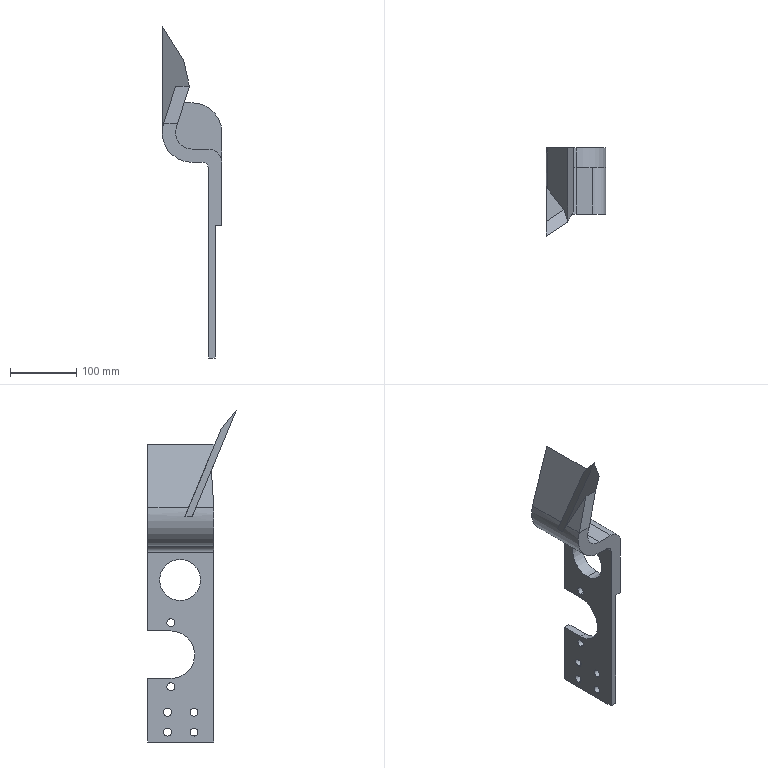Part | SolidWorks | features ICE 13, Extrusion 1, HoleWzd 1 | 1 solid | 65 faces | box 90 x 133.847 x 502.101 mm | volume 777902 mm3 | cylinder 32 | plane 25 | cone 8 | commonest cylinder face diameters 12 x12 5 x8 30 x2 62 x2 70 x2 90 x2